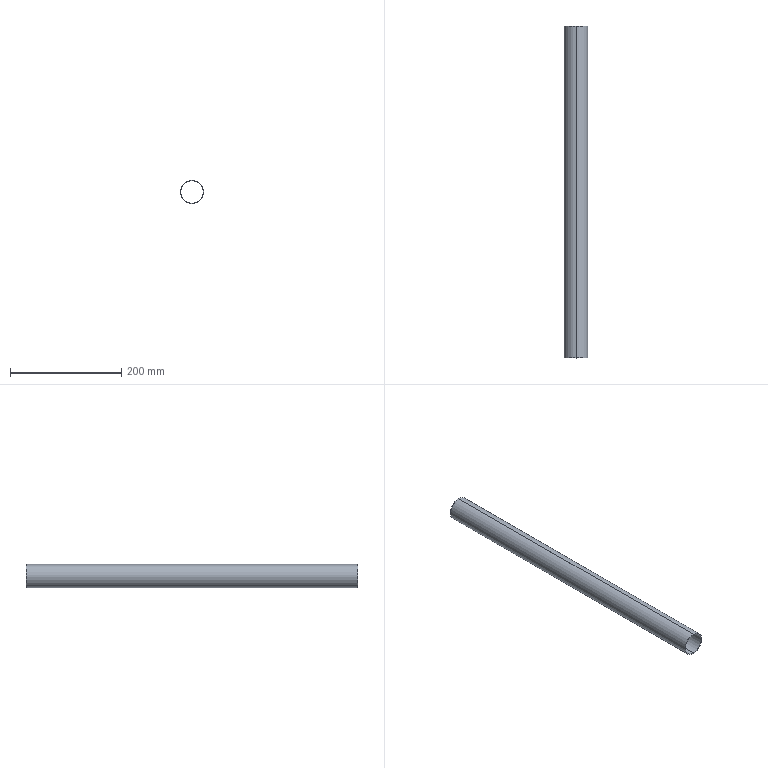Part | SolidWorks | features BaseBody 1 | 1 solid | 6 faces | box 42.16 x 598 x 42.16 mm | volume 62162 mm3 | cylinder 4 | plane 2 | commonest cylinder face diameters 40.56 x2 42.16 x2
STEP:
#1=CARTESIAN_POINT('',(0.,598.,-21.08));
#2=VERTEX_POINT('',#1);
#3=CARTESIAN_POINT('',(0.,598.,21.08));
#4=VERTEX_POINT('',#3);
#5=CARTESIAN_POINT('',(0.,598.,0.));
#6=DIRECTION('',(0.,-1.,0.));
#7=DIRECTION('',(0.,0.,-1.));
#8=AXIS2_PLACEMENT_3D('',#5,#6,#7);
#9=CIRCLE('',#8,21.08);
#10=EDGE_CURVE('',#2,#4,#9,.T.);
#11=ORIENTED_EDGE('',*,*,#10,.T.);
#12=CARTESIAN_POINT('',(0.,0.,21.08));
#13=VERTEX_POINT('',#12);
#14=CARTESIAN_POINT('',(0.,598.,21.08));
#15=DIRECTION('',(0.,-1.,0.));
#16=VECTOR('',#15,1000.);
#17=LINE('',#14,#16);
#18=EDGE_CURVE('',#4,#13,#17,.T.);
#19=ORIENTED_EDGE('',*,*,#18,.T.);
#20=CARTESIAN_POINT('',(0.,0.,-21.08));
#21=VERTEX_POINT('',#20);
#22=CARTESIAN_POINT('',(0.,0.,0.));
#23=DIRECTION('',(0.,1.,0.));
#24=DIRECTION('',(0.,0.,-1.));
#25=AXIS2_PLACEMENT_3D('',#22,#23,#24);
#26=CIRCLE('',#25,21.08);
#27=EDGE_CURVE('',#13,#21,#26,.T.);
#28=ORIENTED_EDGE('',*,*,#27,.T.);
#29=CARTESIAN_POINT('',(0.,598.,-21.08));
#30=DIRECTION('',(0.,-1.,0.));
#31=VECTOR('',#30,1000.);
#32=LINE('',#29,#31);
#33=EDGE_CURVE('',#2,#21,#32,.T.);
#34=ORIENTED_EDGE('',*,*,#33,.F.);
#35=EDGE_LOOP('',(#11,#19,#28,#34));
#36=FACE_OUTER_BOUND('',#35,.T.);
#37=CARTESIAN_POINT('',(0.,598.,0.));
#38=DIRECTION('',(0.,-1.,0.));
#39=DIRECTION('',(0.,0.,-1.));
#40=AXIS2_PLACEMENT_3D('',#37,#38,#39);
#41=CYLINDRICAL_SURFACE('',#40,21.08);
#42=ADVANCED_FACE('',(#36),#41,.T.);
#43=CARTESIAN_POINT('',(0.,598.,20.28));
#44=VERTEX_POINT('',#43);
#45=CARTESIAN_POINT('',(0.,598.,-20.28));
#46=VERTEX_POINT('',#45);
#47=CARTESIAN_POINT('',(0.,598.,0.));
#48=DIRECTION('',(0.,-1.,0.));
#49=DIRECTION('',(0.,0.,-1.));
#50=AXIS2_PLACEMENT_3D('',#47,#48,#49);
#51=CIRCLE('',#50,20.28);
#52=EDGE_CURVE('',#44,#46,#51,.T.);
#53=ORIENTED_EDGE('',*,*,#52,.F.);
#54=CARTESIAN_POINT('',(0.,0.,20.28));
#55=VERTEX_POINT('',#54);
#56=CARTESIAN_POINT('',(0.,598.,20.28));
#57=DIRECTION('',(0.,-1.,0.));
#58=VECTOR('',#57,1000.);
#59=LINE('',#56,#58);
#60=EDGE_CURVE('',#44,#55,#59,.T.);
#61=ORIENTED_EDGE('',*,*,#60,.T.);
#62=CARTESIAN_POINT('',(0.,0.,-20.28));
#63=VERTEX_POINT('',#62);
#64=CARTESIAN_POINT('',(0.,0.,0.));
#65=DIRECTION('',(0.,-1.,0.));
#66=DIRECTION('',(0.,0.,-1.));
#67=AXIS2_PLACEMENT_3D('',#64,#65,#66);
#68=CIRCLE('',#67,20.28);
#69=EDGE_CURVE('',#55,#63,#68,.T.);
#70=ORIENTED_EDGE('',*,*,#69,.T.);
#71=CARTESIAN_POINT('',(0.,598.,-20.28));
#72=DIRECTION('',(0.,-1.,0.));
#73=VECTOR('',#72,1000.);
#74=LINE('',#71,#73);
#75=EDGE_CURVE('',#46,#63,#74,.T.);
#76=ORIENTED_EDGE('',*,*,#75,.F.);
#77=EDGE_LOOP('',(#53,#61,#70,#76));
#78=FACE_OUTER_BOUND('',#77,.T.);
#79=CARTESIAN_POINT('',(0.,598.,0.));
#80=DIRECTION('',(0.,-1.,0.));
#81=DIRECTION('',(0.,0.,-1.));
#82=AXIS2_PLACEMENT_3D('',#79,#80,#81);
#83=CYLINDRICAL_SURFACE('',#82,20.28);
#84=ADVANCED_FACE('',(#78),#83,.F.);
#85=ORIENTED_EDGE('',*,*,#18,.F.);
#86=CARTESIAN_POINT('',(0.,598.,0.));
#87=DIRECTION('',(0.,-1.,0.));
#88=DIRECTION('',(0.,0.,-1.));
#89=AXIS2_PLACEMENT_3D('',#86,#87,#88);
#90=CIRCLE('',#89,21.08);
#91=EDGE_CURVE('',#4,#2,#90,.T.);
#92=ORIENTED_EDGE('',*,*,#91,.T.);
#93=ORIENTED_EDGE('',*,*,#33,.T.);
#94=CARTESIAN_POINT('',(0.,0.,0.));
#95=DIRECTION('',(0.,1.,0.));
#96=DIRECTION('',(0.,0.,-1.));
#97=AXIS2_PLACEMENT_3D('',#94,#95,#96);
#98=CIRCLE('',#97,21.08);
#99=EDGE_CURVE('',#21,#13,#98,.T.);
#100=ORIENTED_EDGE('',*,*,#99,.T.);
#101=EDGE_LOOP('',(#85,#92,#93,#100));
#102=FACE_OUTER_BOUND('',#101,.T.);
#103=CARTESIAN_POINT('',(0.,598.,0.));
#104=DIRECTION('',(0.,-1.,0.));
#105=DIRECTION('',(0.,0.,-1.));
#106=AXIS2_PLACEMENT_3D('',#103,#104,#105);
#107=CYLINDRICAL_SURFACE('',#106,21.08);
#108=ADVANCED_FACE('',(#102),#107,.T.);
#109=CARTESIAN_POINT('',(0.,0.,0.));
#110=DIRECTION('',(0.,-1.,0.));
#111=DIRECTION('',(0.,0.,-1.));
#112=AXIS2_PLACEMENT_3D('',#109,#110,#111);
#113=CIRCLE('',#112,20.28);
#114=EDGE_CURVE('',#63,#55,#113,.T.);
#115=ORIENTED_EDGE('',*,*,#114,.F.);
#116=ORIENTED_EDGE('',*,*,#69,.F.);
#117=EDGE_LOOP('',(#115,#116));
#118=FACE_BOUND('',#117,.T.);
#119=ORIENTED_EDGE('',*,*,#99,.F.);
#120=ORIENTED_EDGE('',*,*,#27,.F.);
#121=EDGE_LOOP('',(#119,#120));
#122=FACE_OUTER_BOUND('',#121,.T.);
#123=CARTESIAN_POINT('',(0.,0.,0.));
#124=DIRECTION('',(0.,1.,0.));
#125=DIRECTION('',(0.,0.,1.));
#126=AXIS2_PLACEMENT_3D('',#123,#124,#125);
#127=PLANE('',#126);
#128=ADVANCED_FACE('',(#118,#122),#127,.F.);
#129=CARTESIAN_POINT('',(0.,598.,0.));
#130=DIRECTION('',(0.,-1.,0.));
#131=DIRECTION('',(0.,0.,-1.));
#132=AXIS2_PLACEMENT_3D('',#129,#130,#131);
#133=CIRCLE('',#132,20.28);
#134=EDGE_CURVE('',#46,#44,#133,.T.);
#135=ORIENTED_EDGE('',*,*,#134,.T.);
#136=ORIENTED_EDGE('',*,*,#52,.T.);
#137=EDGE_LOOP('',(#135,#136));
#138=FACE_BOUND('',#137,.T.);
#139=ORIENTED_EDGE('',*,*,#10,.F.);
#140=ORIENTED_EDGE('',*,*,#91,.F.);
#141=EDGE_LOOP('',(#139,#140));
#142=FACE_OUTER_BOUND('',#141,.T.);
#143=CARTESIAN_POINT('',(0.,598.,0.));
#144=DIRECTION('',(0.,1.,0.));
#145=DIRECTION('',(0.,0.,1.));
#146=AXIS2_PLACEMENT_3D('',#143,#144,#145);
#147=PLANE('',#146);
#148=ADVANCED_FACE('',(#138,#142),#147,.T.);
#149=ORIENTED_EDGE('',*,*,#60,.F.);
#150=ORIENTED_EDGE('',*,*,#134,.F.);
#151=ORIENTED_EDGE('',*,*,#75,.T.);
#152=ORIENTED_EDGE('',*,*,#114,.T.);
#153=EDGE_LOOP('',(#149,#150,#151,#152));
#154=FACE_OUTER_BOUND('',#153,.T.);
#155=CARTESIAN_POINT('',(0.,598.,0.));
#156=DIRECTION('',(0.,-1.,0.));
#157=DIRECTION('',(0.,0.,-1.));
#158=AXIS2_PLACEMENT_3D('',#155,#156,#157);
#159=CYLINDRICAL_SURFACE('',#158,20.28);
#160=ADVANCED_FACE('',(#154),#159,.F.);
#161=CLOSED_SHELL('',(#42,#84,#108,#128,#148,#160));
#162=MANIFOLD_SOLID_BREP('',#161);
#163=CARTESIAN_POINT('',(0.,0.,0.));
#164=DIRECTION('',(0.,0.,1.));
#165=DIRECTION('',(1.,0.,0.));
#166=AXIS2_PLACEMENT_3D('',#163,#164,#165);
#167=(LENGTH_UNIT()NAMED_UNIT(*)SI_UNIT(.MILLI.,.METRE.));
#168=UNCERTAINTY_MEASURE_WITH_UNIT(LENGTH_MEASURE(0.00001),#167,'','');
#169=(NAMED_UNIT(*)PLANE_ANGLE_UNIT()SI_UNIT($,.RADIAN.));
#170=(NAMED_UNIT(*)SI_UNIT($,.STERADIAN.)SOLID_ANGLE_UNIT());
#171=(GEOMETRIC_REPRESENTATION_CONTEXT(3)GLOBAL_UNCERTAINTY_ASSIGNED_CONTEXT((#168))GLOBAL_UNIT_ASSIGNED_CONTEXT((#167,#169,#170))REPRESENTATION_CONTEXT('',''));
#172=ADVANCED_BREP_SHAPE_REPRESENTATION('',(#162,#166),#171);